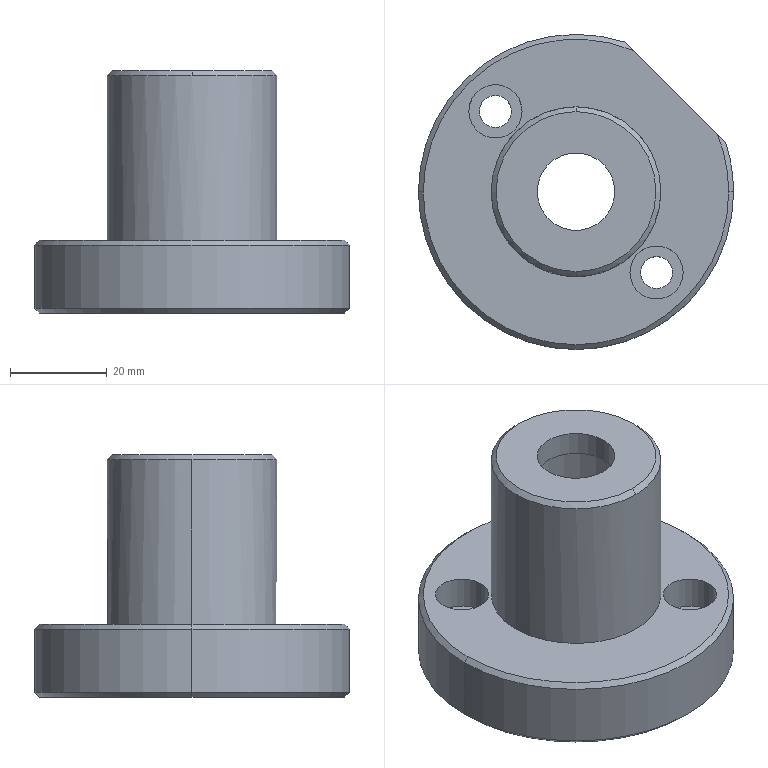Part | STEP file | fBY02F02M-00-14A | 1 solid | 41 faces | box 65 x 65 x 50 mm | volume 50405 mm3 | cylinder 23 | plane 10 | cone 8 | commonest cylinder face diameters 6.6 x4 11 x4 28 x4 65 x3 16 x2 29 x2